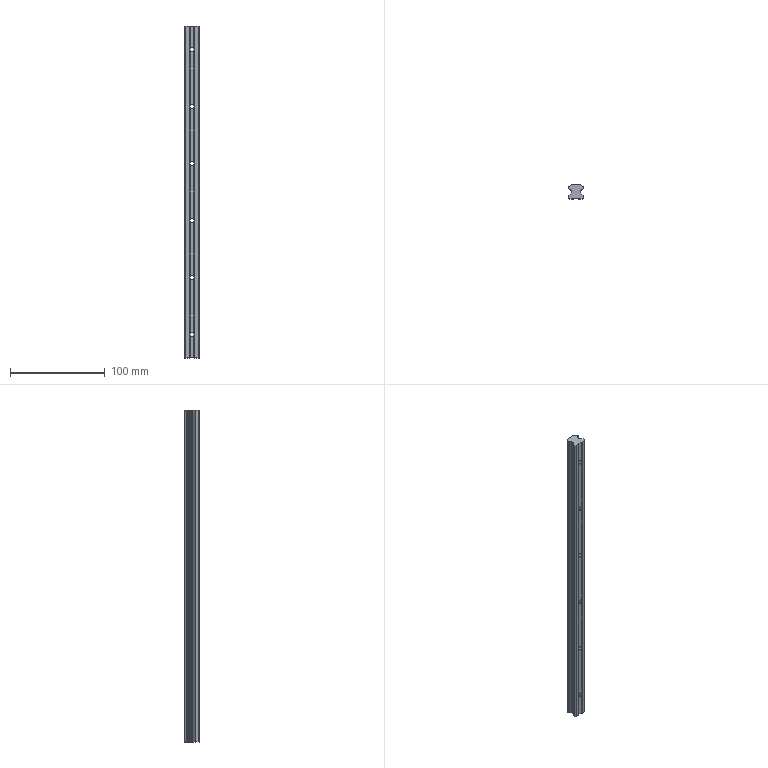Part | SolidWorks | features BaseBody 1 | 1 solid | 74 faces | box 15 x 15 x 350 mm | volume 63532 mm3 | plane 38 | cylinder 36 | commonest cylinder face diameters 4.5 x12 7.5 x12 0.8 x8 3.24 x4